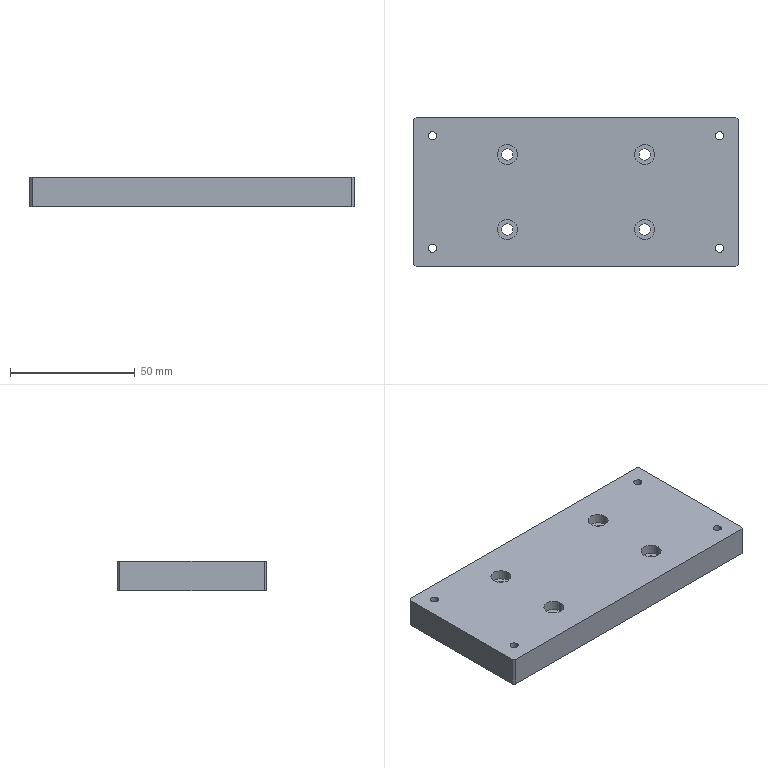Part | NX | features BREP 1 | 1 solid | 38 faces | box 130 x 60 x 12 mm | volume 91852 mm3 | cylinder 24 | plane 14 | commonest cylinder face diameters 3.3 x8 4.5 x8 8 x8
STEP:
#1=CARTESIAN_POINT('',(-59.15,22.5,-6.));
#2=VERTEX_POINT('',#1);
#3=CARTESIAN_POINT('',(-55.85,22.5,-6.));
#4=VERTEX_POINT('',#3);
#5=CARTESIAN_POINT('',(-57.5,22.5,-6.));
#6=DIRECTION('',(0.,0.,1.));
#7=DIRECTION('',(1.,0.,0.));
#8=AXIS2_PLACEMENT_3D('',#5,#6,#7);
#9=CIRCLE('',#8,1.65);
#10=EDGE_CURVE('',#2,#4,#9,.T.);
#11=ORIENTED_EDGE('',*,*,#10,.F.);
#12=CARTESIAN_POINT('',(-59.15,22.5,6.));
#13=VERTEX_POINT('',#12);
#14=CARTESIAN_POINT('',(-59.15,22.5,6.));
#15=DIRECTION('',(0.,0.,1.));
#16=VECTOR('',#15,1000.);
#17=LINE('',#14,#16);
#18=EDGE_CURVE('',#13,#2,#17,.F.);
#19=ORIENTED_EDGE('',*,*,#18,.F.);
#20=CARTESIAN_POINT('',(-55.85,22.5,6.));
#21=VERTEX_POINT('',#20);
#22=CARTESIAN_POINT('',(-57.5,22.5,6.));
#23=DIRECTION('',(0.,0.,1.));
#24=DIRECTION('',(1.,0.,0.));
#25=AXIS2_PLACEMENT_3D('',#22,#23,#24);
#26=CIRCLE('',#25,1.65);
#27=EDGE_CURVE('',#13,#21,#26,.T.);
#28=ORIENTED_EDGE('',*,*,#27,.T.);
#29=CARTESIAN_POINT('',(-55.85,22.5,6.));
#30=DIRECTION('',(0.,0.,1.));
#31=VECTOR('',#30,1000.);
#32=LINE('',#29,#31);
#33=EDGE_CURVE('',#21,#4,#32,.F.);
#34=ORIENTED_EDGE('',*,*,#33,.T.);
#35=EDGE_LOOP('',(#11,#19,#28,#34));
#36=FACE_BOUND('',#35,.T.);
#37=CARTESIAN_POINT('',(-57.5,22.5,6.));
#38=DIRECTION('',(0.,0.,1.));
#39=DIRECTION('',(1.,0.,0.));
#40=AXIS2_PLACEMENT_3D('',#37,#38,#39);
#41=CYLINDRICAL_SURFACE('',#40,1.65);
#42=ADVANCED_FACE('',(#36),#41,.F.);
#43=CARTESIAN_POINT('',(55.85,22.5,-6.));
#44=VERTEX_POINT('',#43);
#45=CARTESIAN_POINT('',(59.15,22.5,-6.));
#46=VERTEX_POINT('',#45);
#47=CARTESIAN_POINT('',(57.5,22.5,-6.));
#48=DIRECTION('',(0.,0.,1.));
#49=DIRECTION('',(1.,0.,0.));
#50=AXIS2_PLACEMENT_3D('',#47,#48,#49);
#51=CIRCLE('',#50,1.65);
#52=EDGE_CURVE('',#44,#46,#51,.T.);
#53=ORIENTED_EDGE('',*,*,#52,.F.);
#54=CARTESIAN_POINT('',(55.85,22.5,6.));
#55=VERTEX_POINT('',#54);
#56=CARTESIAN_POINT('',(55.85,22.5,6.));
#57=DIRECTION('',(0.,0.,1.));
#58=VECTOR('',#57,1000.);
#59=LINE('',#56,#58);
#60=EDGE_CURVE('',#55,#44,#59,.F.);
#61=ORIENTED_EDGE('',*,*,#60,.F.);
#62=CARTESIAN_POINT('',(59.15,22.5,6.));
#63=VERTEX_POINT('',#62);
#64=CARTESIAN_POINT('',(57.5,22.5,6.));
#65=DIRECTION('',(0.,0.,1.));
#66=DIRECTION('',(1.,0.,0.));
#67=AXIS2_PLACEMENT_3D('',#64,#65,#66);
#68=CIRCLE('',#67,1.65);
#69=EDGE_CURVE('',#55,#63,#68,.T.);
#70=ORIENTED_EDGE('',*,*,#69,.T.);
#71=CARTESIAN_POINT('',(59.15,22.5,6.));
#72=DIRECTION('',(0.,0.,1.));
#73=VECTOR('',#72,1000.);
#74=LINE('',#71,#73);
#75=EDGE_CURVE('',#63,#46,#74,.F.);
#76=ORIENTED_EDGE('',*,*,#75,.T.);
#77=EDGE_LOOP('',(#53,#61,#70,#76));
#78=FACE_BOUND('',#77,.T.);
#79=CARTESIAN_POINT('',(57.5,22.5,6.));
#80=DIRECTION('',(0.,0.,1.));
#81=DIRECTION('',(1.,0.,0.));
#82=AXIS2_PLACEMENT_3D('',#79,#80,#81);
#83=CYLINDRICAL_SURFACE('',#82,1.65);
#84=ADVANCED_FACE('',(#78),#83,.F.);
#85=CARTESIAN_POINT('',(-59.15,-22.5,-6.));
#86=VERTEX_POINT('',#85);
#87=CARTESIAN_POINT('',(-55.85,-22.5,-6.));
#88=VERTEX_POINT('',#87);
#89=CARTESIAN_POINT('',(-57.5,-22.5,-6.));
#90=DIRECTION('',(0.,0.,1.));
#91=DIRECTION('',(1.,0.,0.));
#92=AXIS2_PLACEMENT_3D('',#89,#90,#91);
#93=CIRCLE('',#92,1.65);
#94=EDGE_CURVE('',#86,#88,#93,.T.);
#95=ORIENTED_EDGE('',*,*,#94,.F.);
#96=CARTESIAN_POINT('',(-59.15,-22.5,6.));
#97=VERTEX_POINT('',#96);
#98=CARTESIAN_POINT('',(-59.15,-22.5,6.));
#99=DIRECTION('',(0.,0.,1.));
#100=VECTOR('',#99,1000.);
#101=LINE('',#98,#100);
#102=EDGE_CURVE('',#97,#86,#101,.F.);
#103=ORIENTED_EDGE('',*,*,#102,.F.);
#104=CARTESIAN_POINT('',(-55.85,-22.5,6.));
#105=VERTEX_POINT('',#104);
#106=CARTESIAN_POINT('',(-57.5,-22.5,6.));
#107=DIRECTION('',(0.,0.,1.));
#108=DIRECTION('',(1.,0.,0.));
#109=AXIS2_PLACEMENT_3D('',#106,#107,#108);
#110=CIRCLE('',#109,1.65);
#111=EDGE_CURVE('',#97,#105,#110,.T.);
#112=ORIENTED_EDGE('',*,*,#111,.T.);
#113=CARTESIAN_POINT('',(-55.85,-22.5,6.));
#114=DIRECTION('',(0.,0.,1.));
#115=VECTOR('',#114,1000.);
#116=LINE('',#113,#115);
#117=EDGE_CURVE('',#105,#88,#116,.F.);
#118=ORIENTED_EDGE('',*,*,#117,.T.);
#119=EDGE_LOOP('',(#95,#103,#112,#118));
#120=FACE_BOUND('',#119,.T.);
#121=CARTESIAN_POINT('',(-57.5,-22.5,6.));
#122=DIRECTION('',(0.,0.,1.));
#123=DIRECTION('',(1.,0.,0.));
#124=AXIS2_PLACEMENT_3D('',#121,#122,#123);
#125=CYLINDRICAL_SURFACE('',#124,1.65);
#126=ADVANCED_FACE('',(#120),#125,.F.);
#127=CARTESIAN_POINT('',(55.85,-22.5,-6.));
#128=VERTEX_POINT('',#127);
#129=CARTESIAN_POINT('',(59.15,-22.5,-6.));
#130=VERTEX_POINT('',#129);
#131=CARTESIAN_POINT('',(57.5,-22.5,-6.));
#132=DIRECTION('',(0.,0.,1.));
#133=DIRECTION('',(1.,0.,0.));
#134=AXIS2_PLACEMENT_3D('',#131,#132,#133);
#135=CIRCLE('',#134,1.65);
#136=EDGE_CURVE('',#128,#130,#135,.T.);
#137=ORIENTED_EDGE('',*,*,#136,.F.);
#138=CARTESIAN_POINT('',(55.85,-22.5,6.));
#139=VERTEX_POINT('',#138);
#140=CARTESIAN_POINT('',(55.85,-22.5,6.));
#141=DIRECTION('',(0.,0.,1.));
#142=VECTOR('',#141,1000.);
#143=LINE('',#140,#142);
#144=EDGE_CURVE('',#139,#128,#143,.F.);
#145=ORIENTED_EDGE('',*,*,#144,.F.);
#146=CARTESIAN_POINT('',(59.15,-22.5,6.));
#147=VERTEX_POINT('',#146);
#148=CARTESIAN_POINT('',(57.5,-22.5,6.));
#149=DIRECTION('',(0.,0.,1.));
#150=DIRECTION('',(1.,0.,0.));
#151=AXIS2_PLACEMENT_3D('',#148,#149,#150);
#152=CIRCLE('',#151,1.65);
#153=EDGE_CURVE('',#139,#147,#152,.T.);
#154=ORIENTED_EDGE('',*,*,#153,.T.);
#155=CARTESIAN_POINT('',(59.15,-22.5,6.));
#156=DIRECTION('',(0.,0.,1.));
#157=VECTOR('',#156,1000.);
#158=LINE('',#155,#157);
#159=EDGE_CURVE('',#147,#130,#158,.F.);
#160=ORIENTED_EDGE('',*,*,#159,.T.);
#161=EDGE_LOOP('',(#137,#145,#154,#160));
#162=FACE_BOUND('',#161,.T.);
#163=CARTESIAN_POINT('',(57.5,-22.5,6.));
#164=DIRECTION('',(0.,0.,1.));
#165=DIRECTION('',(1.,0.,0.));
#166=AXIS2_PLACEMENT_3D('',#163,#164,#165);
#167=CYLINDRICAL_SURFACE('',#166,1.65);
#168=ADVANCED_FACE('',(#162),#167,.F.);
#169=CARTESIAN_POINT('',(-31.5,15.,2.));
#170=VERTEX_POINT('',#169);
#171=CARTESIAN_POINT('',(-23.5,15.,2.));
#172=VERTEX_POINT('',#171);
#173=CARTESIAN_POINT('',(-27.5,15.,2.));
#174=DIRECTION('',(0.,0.,1.));
#175=DIRECTION('',(1.,0.,0.));
#176=AXIS2_PLACEMENT_3D('',#173,#174,#175);
#177=CIRCLE('',#176,4.);
#178=EDGE_CURVE('',#170,#172,#177,.T.);
#179=ORIENTED_EDGE('',*,*,#178,.F.);
#180=CARTESIAN_POINT('',(-31.5,15.,6.));
#181=VERTEX_POINT('',#180);
#182=CARTESIAN_POINT('',(-31.5,15.,6.));
#183=DIRECTION('',(0.,0.,1.));
#184=VECTOR('',#183,1000.);
#185=LINE('',#182,#184);
#186=EDGE_CURVE('',#181,#170,#185,.F.);
#187=ORIENTED_EDGE('',*,*,#186,.F.);
#188=CARTESIAN_POINT('',(-23.5,15.,6.));
#189=VERTEX_POINT('',#188);
#190=CARTESIAN_POINT('',(-27.5,15.,6.));
#191=DIRECTION('',(0.,0.,1.));
#192=DIRECTION('',(1.,0.,0.));
#193=AXIS2_PLACEMENT_3D('',#190,#191,#192);
#194=CIRCLE('',#193,4.);
#195=EDGE_CURVE('',#181,#189,#194,.T.);
#196=ORIENTED_EDGE('',*,*,#195,.T.);
#197=CARTESIAN_POINT('',(-23.5,15.,6.));
#198=DIRECTION('',(0.,0.,1.));
#199=VECTOR('',#198,1000.);
#200=LINE('',#197,#199);
#201=EDGE_CURVE('',#189,#172,#200,.F.);
#202=ORIENTED_EDGE('',*,*,#201,.T.);
#203=EDGE_LOOP('',(#179,#187,#196,#202));
#204=FACE_BOUND('',#203,.T.);
#205=CARTESIAN_POINT('',(-27.5,15.,6.));
#206=DIRECTION('',(0.,0.,1.));
#207=DIRECTION('',(1.,0.,0.));
#208=AXIS2_PLACEMENT_3D('',#205,#206,#207);
#209=CYLINDRICAL_SURFACE('',#208,4.);
#210=ADVANCED_FACE('',(#204),#209,.F.);
#211=CARTESIAN_POINT('',(-29.75,15.,-6.));
#212=VERTEX_POINT('',#211);
#213=CARTESIAN_POINT('',(-25.25,15.,-6.));
#214=VERTEX_POINT('',#213);
#215=CARTESIAN_POINT('',(-27.5,15.,-6.));
#216=DIRECTION('',(0.,0.,1.));
#217=DIRECTION('',(1.,0.,0.));
#218=AXIS2_PLACEMENT_3D('',#215,#216,#217);
#219=CIRCLE('',#218,2.25);
#220=EDGE_CURVE('',#212,#214,#219,.T.);
#221=ORIENTED_EDGE('',*,*,#220,.F.);
#222=CARTESIAN_POINT('',(-29.75,15.,2.));
#223=VERTEX_POINT('',#222);
#224=CARTESIAN_POINT('',(-29.75,15.,6.));
#225=DIRECTION('',(0.,0.,1.));
#226=VECTOR('',#225,1000.);
#227=LINE('',#224,#226);
#228=EDGE_CURVE('',#223,#212,#227,.F.);
#229=ORIENTED_EDGE('',*,*,#228,.F.);
#230=CARTESIAN_POINT('',(-25.25,15.,2.));
#231=VERTEX_POINT('',#230);
#232=CARTESIAN_POINT('',(-27.5,15.,2.));
#233=DIRECTION('',(0.,0.,1.));
#234=DIRECTION('',(1.,0.,0.));
#235=AXIS2_PLACEMENT_3D('',#232,#233,#234);
#236=CIRCLE('',#235,2.25);
#237=EDGE_CURVE('',#223,#231,#236,.T.);
#238=ORIENTED_EDGE('',*,*,#237,.T.);
#239=CARTESIAN_POINT('',(-25.25,15.,6.));
#240=DIRECTION('',(0.,0.,1.));
#241=VECTOR('',#240,1000.);
#242=LINE('',#239,#241);
#243=EDGE_CURVE('',#231,#214,#242,.F.);
#244=ORIENTED_EDGE('',*,*,#243,.T.);
#245=EDGE_LOOP('',(#221,#229,#238,#244));
#246=FACE_BOUND('',#245,.T.);
#247=CARTESIAN_POINT('',(-27.5,15.,6.));
#248=DIRECTION('',(0.,0.,1.));
#249=DIRECTION('',(1.,0.,0.));
#250=AXIS2_PLACEMENT_3D('',#247,#248,#249);
#251=CYLINDRICAL_SURFACE('',#250,2.25);
#252=ADVANCED_FACE('',(#246),#251,.F.);
#253=CARTESIAN_POINT('',(23.5,15.,2.));
#254=VERTEX_POINT('',#253);
#255=CARTESIAN_POINT('',(31.5,15.,2.));
#256=VERTEX_POINT('',#255);
#257=CARTESIAN_POINT('',(27.5,15.,2.));
#258=DIRECTION('',(0.,0.,1.));
#259=DIRECTION('',(1.,0.,0.));
#260=AXIS2_PLACEMENT_3D('',#257,#258,#259);
#261=CIRCLE('',#260,4.);
#262=EDGE_CURVE('',#254,#256,#261,.T.);
#263=ORIENTED_EDGE('',*,*,#262,.F.);
#264=CARTESIAN_POINT('',(23.5,15.,6.));
#265=VERTEX_POINT('',#264);
#266=CARTESIAN_POINT('',(23.5,15.,6.));
#267=DIRECTION('',(0.,0.,1.));
#268=VECTOR('',#267,1000.);
#269=LINE('',#266,#268);
#270=EDGE_CURVE('',#265,#254,#269,.F.);
#271=ORIENTED_EDGE('',*,*,#270,.F.);
#272=CARTESIAN_POINT('',(31.5,15.,6.));
#273=VERTEX_POINT('',#272);
#274=CARTESIAN_POINT('',(27.5,15.,6.));
#275=DIRECTION('',(0.,0.,1.));
#276=DIRECTION('',(1.,0.,0.));
#277=AXIS2_PLACEMENT_3D('',#274,#275,#276);
#278=CIRCLE('',#277,4.);
#279=EDGE_CURVE('',#265,#273,#278,.T.);
#280=ORIENTED_EDGE('',*,*,#279,.T.);
#281=CARTESIAN_POINT('',(31.5,15.,6.));
#282=DIRECTION('',(0.,0.,1.));
#283=VECTOR('',#282,1000.);
#284=LINE('',#281,#283);
#285=EDGE_CURVE('',#273,#256,#284,.F.);
#286=ORIENTED_EDGE('',*,*,#285,.T.);
#287=EDGE_LOOP('',(#263,#271,#280,#286));
#288=FACE_BOUND('',#287,.T.);
#289=CARTESIAN_POINT('',(27.5,15.,6.));
#290=DIRECTION('',(0.,0.,1.));
#291=DIRECTION('',(1.,0.,0.));
#292=AXIS2_PLACEMENT_3D('',#289,#290,#291);
#293=CYLINDRICAL_SURFACE('',#292,4.);
#294=ADVANCED_FACE('',(#288),#293,.F.);
#295=CARTESIAN_POINT('',(25.25,15.,-6.));
#296=VERTEX_POINT('',#295);
#297=CARTESIAN_POINT('',(29.75,15.,-6.));
#298=VERTEX_POINT('',#297);
#299=CARTESIAN_POINT('',(27.5,15.,-6.));
#300=DIRECTION('',(0.,0.,1.));
#301=DIRECTION('',(1.,0.,0.));
#302=AXIS2_PLACEMENT_3D('',#299,#300,#301);
#303=CIRCLE('',#302,2.25);
#304=EDGE_CURVE('',#296,#298,#303,.T.);
#305=ORIENTED_EDGE('',*,*,#304,.F.);
#306=CARTESIAN_POINT('',(25.25,15.,2.));
#307=VERTEX_POINT('',#306);
#308=CARTESIAN_POINT('',(25.25,15.,6.));
#309=DIRECTION('',(0.,0.,1.));
#310=VECTOR('',#309,1000.);
#311=LINE('',#308,#310);
#312=EDGE_CURVE('',#307,#296,#311,.F.);
#313=ORIENTED_EDGE('',*,*,#312,.F.);
#314=CARTESIAN_POINT('',(29.75,15.,2.));
#315=VERTEX_POINT('',#314);
#316=CARTESIAN_POINT('',(27.5,15.,2.));
#317=DIRECTION('',(0.,0.,1.));
#318=DIRECTION('',(1.,0.,0.));
#319=AXIS2_PLACEMENT_3D('',#316,#317,#318);
#320=CIRCLE('',#319,2.25);
#321=EDGE_CURVE('',#307,#315,#320,.T.);
#322=ORIENTED_EDGE('',*,*,#321,.T.);
#323=CARTESIAN_POINT('',(29.75,15.,6.));
#324=DIRECTION('',(0.,0.,1.));
#325=VECTOR('',#324,1000.);
#326=LINE('',#323,#325);
#327=EDGE_CURVE('',#315,#298,#326,.F.);
#328=ORIENTED_EDGE('',*,*,#327,.T.);
#329=EDGE_LOOP('',(#305,#313,#322,#328));
#330=FACE_BOUND('',#329,.T.);
#331=CARTESIAN_POINT('',(27.5,15.,6.));
#332=DIRECTION('',(0.,0.,1.));
#333=DIRECTION('',(1.,0.,0.));
#334=AXIS2_PLACEMENT_3D('',#331,#332,#333);
#335=CYLINDRICAL_SURFACE('',#334,2.25);
#336=ADVANCED_FACE('',(#330),#335,.F.);
#337=CARTESIAN_POINT('',(-31.5,-15.,2.));
#338=VERTEX_POINT('',#337);
#339=CARTESIAN_POINT('',(-23.5,-15.,2.));
#340=VERTEX_POINT('',#339);
#341=CARTESIAN_POINT('',(-27.5,-15.,2.));
#342=DIRECTION('',(0.,0.,1.));
#343=DIRECTION('',(1.,0.,0.));
#344=AXIS2_PLACEMENT_3D('',#341,#342,#343);
#345=CIRCLE('',#344,4.);
#346=EDGE_CURVE('',#338,#340,#345,.T.);
#347=ORIENTED_EDGE('',*,*,#346,.F.);
#348=CARTESIAN_POINT('',(-31.5,-15.,6.));
#349=VERTEX_POINT('',#348);
#350=CARTESIAN_POINT('',(-31.5,-15.,6.));
#351=DIRECTION('',(0.,0.,1.));
#352=VECTOR('',#351,1000.);
#353=LINE('',#350,#352);
#354=EDGE_CURVE('',#349,#338,#353,.F.);
#355=ORIENTED_EDGE('',*,*,#354,.F.);
#356=CARTESIAN_POINT('',(-23.5,-15.,6.));
#357=VERTEX_POINT('',#356);
#358=CARTESIAN_POINT('',(-27.5,-15.,6.));
#359=DIRECTION('',(0.,0.,1.));
#360=DIRECTION('',(1.,0.,0.));
#361=AXIS2_PLACEMENT_3D('',#358,#359,#360);
#362=CIRCLE('',#361,4.);
#363=EDGE_CURVE('',#349,#357,#362,.T.);
#364=ORIENTED_EDGE('',*,*,#363,.T.);
#365=CARTESIAN_POINT('',(-23.5,-15.,6.));
#366=DIRECTION('',(0.,0.,1.));
#367=VECTOR('',#366,1000.);
#368=LINE('',#365,#367);
#369=EDGE_CURVE('',#357,#340,#368,.F.);
#370=ORIENTED_EDGE('',*,*,#369,.T.);
#371=EDGE_LOOP('',(#347,#355,#364,#370));
#372=FACE_BOUND('',#371,.T.);
#373=CARTESIAN_POINT('',(-27.5,-15.,6.));
#374=DIRECTION('',(0.,0.,1.));
#375=DIRECTION('',(1.,0.,0.));
#376=AXIS2_PLACEMENT_3D('',#373,#374,#375);
#377=CYLINDRICAL_SURFACE('',#376,4.);
#378=ADVANCED_FACE('',(#372),#377,.F.);
#379=CARTESIAN_POINT('',(-29.75,-15.,-6.));
#380=VERTEX_POINT('',#379);
#381=CARTESIAN_POINT('',(-25.25,-15.,-6.));
#382=VERTEX_POINT('',#381);
#383=CARTESIAN_POINT('',(-27.5,-15.,-6.));
#384=DIRECTION('',(0.,0.,1.));
#385=DIRECTION('',(1.,0.,0.));
#386=AXIS2_PLACEMENT_3D('',#383,#384,#385);
#387=CIRCLE('',#386,2.25);
#388=EDGE_CURVE('',#380,#382,#387,.T.);
#389=ORIENTED_EDGE('',*,*,#388,.F.);
#390=CARTESIAN_POINT('',(-29.75,-15.,2.));
#391=VERTEX_POINT('',#390);
#392=CARTESIAN_POINT('',(-29.75,-15.,6.));
#393=DIRECTION('',(0.,0.,1.));
#394=VECTOR('',#393,1000.);
#395=LINE('',#392,#394);
#396=EDGE_CURVE('',#391,#380,#395,.F.);
#397=ORIENTED_EDGE('',*,*,#396,.F.);
#398=CARTESIAN_POINT('',(-25.25,-15.,2.));
#399=VERTEX_POINT('',#398);
#400=CARTESIAN_POINT('',(-27.5,-15.,2.));
#401=DIRECTION('',(0.,0.,1.));
#402=DIRECTION('',(1.,0.,0.));
#403=AXIS2_PLACEMENT_3D('',#400,#401,#402);
#404=CIRCLE('',#403,2.25);
#405=EDGE_CURVE('',#391,#399,#404,.T.);
#406=ORIENTED_EDGE('',*,*,#405,.T.);
#407=CARTESIAN_POINT('',(-25.25,-15.,6.));
#408=DIRECTION('',(0.,0.,1.));
#409=VECTOR('',#408,1000.);
#410=LINE('',#407,#409);
#411=EDGE_CURVE('',#399,#382,#410,.F.);
#412=ORIENTED_EDGE('',*,*,#411,.T.);
#413=EDGE_LOOP('',(#389,#397,#406,#412));
#414=FACE_BOUND('',#413,.T.);
#415=CARTESIAN_POINT('',(-27.5,-15.,6.));
#416=DIRECTION('',(0.,0.,1.));
#417=DIRECTION('',(1.,0.,0.));
#418=AXIS2_PLACEMENT_3D('',#415,#416,#417);
#419=CYLINDRICAL_SURFACE('',#418,2.25);
#420=ADVANCED_FACE('',(#414),#419,.F.);
#421=CARTESIAN_POINT('',(23.5,-15.,2.));
#422=VERTEX_POINT('',#421);
#423=CARTESIAN_POINT('',(31.5,-15.,2.));
#424=VERTEX_POINT('',#423);
#425=CARTESIAN_POINT('',(27.5,-15.,2.));
#426=DIRECTION('',(0.,0.,1.));
#427=DIRECTION('',(1.,0.,0.));
#428=AXIS2_PLACEMENT_3D('',#425,#426,#427);
#429=CIRCLE('',#428,4.);
#430=EDGE_CURVE('',#422,#424,#429,.T.);
#431=ORIENTED_EDGE('',*,*,#430,.F.);
#432=CARTESIAN_POINT('',(23.5,-15.,6.));
#433=VERTEX_POINT('',#432);
#434=CARTESIAN_POINT('',(23.5,-15.,6.));
#435=DIRECTION('',(0.,0.,1.));
#436=VECTOR('',#435,1000.);
#437=LINE('',#434,#436);
#438=EDGE_CURVE('',#433,#422,#437,.F.);
#439=ORIENTED_EDGE('',*,*,#438,.F.);
#440=CARTESIAN_POINT('',(31.5,-15.,6.));
#441=VERTEX_POINT('',#440);
#442=CARTESIAN_POINT('',(27.5,-15.,6.));
#443=DIRECTION('',(0.,0.,1.));
#444=DIRECTION('',(1.,0.,0.));
#445=AXIS2_PLACEMENT_3D('',#442,#443,#444);
#446=CIRCLE('',#445,4.);
#447=EDGE_CURVE('',#433,#441,#446,.T.);
#448=ORIENTED_EDGE('',*,*,#447,.T.);
#449=CARTESIAN_POINT('',(31.5,-15.,6.));
#450=DIRECTION('',(0.,0.,1.));
#451=VECTOR('',#450,1000.);
#452=LINE('',#449,#451);
#453=EDGE_CURVE('',#441,#424,#452,.F.);
#454=ORIENTED_EDGE('',*,*,#453,.T.);
#455=EDGE_LOOP('',(#431,#439,#448,#454));
#456=FACE_BOUND('',#455,.T.);
#457=CARTESIAN_POINT('',(27.5,-15.,6.));
#458=DIRECTION('',(0.,0.,1.));
#459=DIRECTION('',(1.,0.,0.));
#460=AXIS2_PLACEMENT_3D('',#457,#458,#459);
#461=CYLINDRICAL_SURFACE('',#460,4.);
#462=ADVANCED_FACE('',(#456),#461,.F.);
#463=CARTESIAN_POINT('',(25.25,-15.,-6.));
#464=VERTEX_POINT('',#463);
#465=CARTESIAN_POINT('',(29.75,-15.,-6.));
#466=VERTEX_POINT('',#465);
#467=CARTESIAN_POINT('',(27.5,-15.,-6.));
#468=DIRECTION('',(0.,0.,1.));
#469=DIRECTION('',(1.,0.,0.));
#470=AXIS2_PLACEMENT_3D('',#467,#468,#469);
#471=CIRCLE('',#470,2.25);
#472=EDGE_CURVE('',#464,#466,#471,.T.);
#473=ORIENTED_EDGE('',*,*,#472,.F.);
#474=CARTESIAN_POINT('',(25.25,-15.,2.));
#475=VERTEX_POINT('',#474);
#476=CARTESIAN_POINT('',(25.25,-15.,6.));
#477=DIRECTION('',(0.,0.,1.));
#478=VECTOR('',#477,1000.);
#479=LINE('',#476,#478);
#480=EDGE_CURVE('',#475,#464,#479,.F.);
#481=ORIENTED_EDGE('',*,*,#480,.F.);
#482=CARTESIAN_POINT('',(29.75,-15.,2.));
#483=VERTEX_POINT('',#482);
#484=CARTESIAN_POINT('',(27.5,-15.,2.));
#485=DIRECTION('',(0.,0.,1.));
#486=DIRECTION('',(1.,0.,0.));
#487=AXIS2_PLACEMENT_3D('',#484,#485,#486);
#488=CIRCLE('',#487,2.25);
#489=EDGE_CURVE('',#475,#483,#488,.T.);
#490=ORIENTED_EDGE('',*,*,#489,.T.);
#491=CARTESIAN_POINT('',(29.75,-15.,6.));
#492=DIRECTION('',(0.,0.,1.));
#493=VECTOR('',#492,1000.);
#494=LINE('',#491,#493);
#495=EDGE_CURVE('',#483,#466,#494,.F.);
#496=ORIENTED_EDGE('',*,*,#495,.T.);
#497=EDGE_LOOP('',(#473,#481,#490,#496));
#498=FACE_BOUND('',#497,.T.);
#499=CARTESIAN_POINT('',(27.5,-15.,6.));
#500=DIRECTION('',(0.,0.,1.));
#501=DIRECTION('',(1.,0.,0.));
#502=AXIS2_PLACEMENT_3D('',#499,#500,#501);
#503=CYLINDRICAL_SURFACE('',#502,2.25);
#504=ADVANCED_FACE('',(#498),#503,.F.);
#505=CARTESIAN_POINT('',(-65.,29.,-6.));
#506=VERTEX_POINT('',#505);
#507=CARTESIAN_POINT('',(-65.,-29.,-6.));
#508=VERTEX_POINT('',#507);
#509=CARTESIAN_POINT('',(-65.,-30.,-6.));
#510=DIRECTION('',(0.,-1.,0.));
#511=VECTOR('',#510,1000.);
#512=LINE('',#509,#511);
#513=EDGE_CURVE('',#506,#508,#512,.T.);
#514=ORIENTED_EDGE('',*,*,#513,.T.);
#515=CARTESIAN_POINT('',(-65.,-29.,6.));
#516=VERTEX_POINT('',#515);
#517=CARTESIAN_POINT('',(-65.,-29.,6.));
#518=DIRECTION('',(0.,0.,1.));
#519=VECTOR('',#518,1000.);
#520=LINE('',#517,#519);
#521=EDGE_CURVE('',#508,#516,#520,.T.);
#522=ORIENTED_EDGE('',*,*,#521,.T.);
#523=CARTESIAN_POINT('',(-65.,29.,6.));
#524=VERTEX_POINT('',#523);
#525=CARTESIAN_POINT('',(-65.,-30.,6.));
#526=DIRECTION('',(0.,-1.,0.));
#527=VECTOR('',#526,1000.);
#528=LINE('',#525,#527);
#529=EDGE_CURVE('',#524,#516,#528,.T.);
#530=ORIENTED_EDGE('',*,*,#529,.F.);
#531=CARTESIAN_POINT('',(-65.,29.,6.));
#532=DIRECTION('',(0.,0.,-1.));
#533=VECTOR('',#532,1000.);
#534=LINE('',#531,#533);
#535=EDGE_CURVE('',#524,#506,#534,.T.);
#536=ORIENTED_EDGE('',*,*,#535,.T.);
#537=EDGE_LOOP('',(#514,#522,#530,#536));
#538=FACE_BOUND('',#537,.T.);
#539=CARTESIAN_POINT('',(-65.,-30.,6.));
#540=DIRECTION('',(1.,0.,0.));
#541=DIRECTION('',(0.,1.,0.));
#542=AXIS2_PLACEMENT_3D('',#539,#540,#541);
#543=PLANE('',#542);
#544=ADVANCED_FACE('',(#538),#543,.F.);
#545=CARTESIAN_POINT('',(-64.,-30.,6.));
#546=VERTEX_POINT('',#545);
#547=CARTESIAN_POINT('',(64.,-30.,6.));
#548=VERTEX_POINT('',#547);
#549=CARTESIAN_POINT('',(65.,-30.,6.));
#550=DIRECTION('',(1.,0.,0.));
#551=VECTOR('',#550,1000.);
#552=LINE('',#549,#551);
#553=EDGE_CURVE('',#546,#548,#552,.T.);
#554=ORIENTED_EDGE('',*,*,#553,.F.);
#555=CARTESIAN_POINT('',(-64.,-30.,-6.));
#556=VERTEX_POINT('',#555);
#557=CARTESIAN_POINT('',(-64.,-30.,6.));
#558=DIRECTION('',(0.,0.,-1.));
#559=VECTOR('',#558,1000.);
#560=LINE('',#557,#559);
#561=EDGE_CURVE('',#546,#556,#560,.T.);
#562=ORIENTED_EDGE('',*,*,#561,.T.);
#563=CARTESIAN_POINT('',(64.,-30.,-6.));
#564=VERTEX_POINT('',#563);
#565=CARTESIAN_POINT('',(65.,-30.,-6.));
#566=DIRECTION('',(1.,0.,0.));
#567=VECTOR('',#566,1000.);
#568=LINE('',#565,#567);
#569=EDGE_CURVE('',#556,#564,#568,.T.);
#570=ORIENTED_EDGE('',*,*,#569,.T.);
#571=CARTESIAN_POINT('',(64.,-30.,6.));
#572=DIRECTION('',(0.,0.,1.));
#573=VECTOR('',#572,1000.);
#574=LINE('',#571,#573);
#575=EDGE_CURVE('',#564,#548,#574,.T.);
#576=ORIENTED_EDGE('',*,*,#575,.T.);
#577=EDGE_LOOP('',(#554,#562,#570,#576));
#578=FACE_BOUND('',#577,.T.);
#579=CARTESIAN_POINT('',(65.,-30.,6.));
#580=DIRECTION('',(0.,1.,0.));
#581=DIRECTION('',(1.,0.,0.));
#582=AXIS2_PLACEMENT_3D('',#579,#580,#581);
#583=PLANE('',#582);
#584=ADVANCED_FACE('',(#578),#583,.F.);
#585=CARTESIAN_POINT('',(65.,-29.,6.));
#586=VERTEX_POINT('',#585);
#587=CARTESIAN_POINT('',(65.,29.,6.));
#588=VERTEX_POINT('',#587);
#589=CARTESIAN_POINT('',(65.,-30.,6.));
#590=DIRECTION('',(0.,1.,0.));
#591=VECTOR('',#590,1000.);
#592=LINE('',#589,#591);
#593=EDGE_CURVE('',#586,#588,#592,.T.);
#594=ORIENTED_EDGE('',*,*,#593,.F.);
#595=CARTESIAN_POINT('',(65.,-29.,-6.));
#596=VERTEX_POINT('',#595);
#597=CARTESIAN_POINT('',(65.,-29.,6.));
#598=DIRECTION('',(0.,0.,-1.));
#599=VECTOR('',#598,1000.);
#600=LINE('',#597,#599);
#601=EDGE_CURVE('',#586,#596,#600,.T.);
#602=ORIENTED_EDGE('',*,*,#601,.T.);
#603=CARTESIAN_POINT('',(65.,29.,-6.));
#604=VERTEX_POINT('',#603);
#605=CARTESIAN_POINT('',(65.,-30.,-6.));
#606=DIRECTION('',(0.,1.,0.));
#607=VECTOR('',#606,1000.);
#608=LINE('',#605,#607);
#609=EDGE_CURVE('',#596,#604,#608,.T.);
#610=ORIENTED_EDGE('',*,*,#609,.T.);
#611=CARTESIAN_POINT('',(65.,29.,6.));
#612=DIRECTION('',(0.,0.,1.));
#613=VECTOR('',#612,1000.);
#614=LINE('',#611,#613);
#615=EDGE_CURVE('',#604,#588,#614,.T.);
#616=ORIENTED_EDGE('',*,*,#615,.T.);
#617=EDGE_LOOP('',(#594,#602,#610,#616));
#618=FACE_BOUND('',#617,.T.);
#619=CARTESIAN_POINT('',(65.,-30.,6.));
#620=DIRECTION('',(-1.,0.,0.));
#621=DIRECTION('',(0.,0.,1.));
#622=AXIS2_PLACEMENT_3D('',#619,#620,#621);
#623=PLANE('',#622);
#624=ADVANCED_FACE('',(#618),#623,.F.);
#625=CARTESIAN_POINT('',(64.,30.,-6.));
#626=VERTEX_POINT('',#625);
#627=CARTESIAN_POINT('',(-64.,30.,-6.));
#628=VERTEX_POINT('',#627);
#629=CARTESIAN_POINT('',(65.,30.,-6.));
#630=DIRECTION('',(-1.,0.,0.));
#631=VECTOR('',#630,1000.);
#632=LINE('',#629,#631);
#633=EDGE_CURVE('',#626,#628,#632,.T.);
#634=ORIENTED_EDGE('',*,*,#633,.T.);
#635=CARTESIAN_POINT('',(-64.,30.,6.));
#636=VERTEX_POINT('',#635);
#637=CARTESIAN_POINT('',(-64.,30.,6.));
#638=DIRECTION('',(0.,0.,1.));
#639=VECTOR('',#638,1000.);
#640=LINE('',#637,#639);
#641=EDGE_CURVE('',#628,#636,#640,.T.);
#642=ORIENTED_EDGE('',*,*,#641,.T.);
#643=CARTESIAN_POINT('',(64.,30.,6.));
#644=VERTEX_POINT('',#643);
#645=CARTESIAN_POINT('',(65.,30.,6.));
#646=DIRECTION('',(-1.,0.,0.));
#647=VECTOR('',#646,1000.);
#648=LINE('',#645,#647);
#649=EDGE_CURVE('',#644,#636,#648,.T.);
#650=ORIENTED_EDGE('',*,*,#649,.F.);
#651=CARTESIAN_POINT('',(64.,30.,6.));
#652=DIRECTION('',(0.,0.,-1.));
#653=VECTOR('',#652,1000.);
#654=LINE('',#651,#653);
#655=EDGE_CURVE('',#644,#626,#654,.T.);
#656=ORIENTED_EDGE('',*,*,#655,.T.);
#657=EDGE_LOOP('',(#634,#642,#650,#656));
#658=FACE_BOUND('',#657,.T.);
#659=CARTESIAN_POINT('',(65.,30.,6.));
#660=DIRECTION('',(0.,-1.,0.));
#661=DIRECTION('',(0.,0.,-1.));
#662=AXIS2_PLACEMENT_3D('',#659,#660,#661);
#663=PLANE('',#662);
#664=ADVANCED_FACE('',(#658),#663,.F.);
#665=ORIENTED_EDGE('',*,*,#529,.T.);
#666=CARTESIAN_POINT('',(-47.,-47.,6.));
#667=DIRECTION('',(0.7071,-0.7071,0.));
#668=VECTOR('',#667,1000.);
#669=LINE('',#666,#668);
#670=EDGE_CURVE('',#516,#546,#669,.T.);
#671=ORIENTED_EDGE('',*,*,#670,.T.);
#672=ORIENTED_EDGE('',*,*,#553,.T.);
#673=CARTESIAN_POINT('',(47.,-47.,6.));
#674=DIRECTION('',(0.7071,0.7071,0.));
#675=VECTOR('',#674,1000.);
#676=LINE('',#673,#675);
#677=EDGE_CURVE('',#548,#586,#676,.T.);
#678=ORIENTED_EDGE('',*,*,#677,.T.);
#679=ORIENTED_EDGE('',*,*,#593,.T.);
#680=CARTESIAN_POINT('',(47.,47.,6.));
#681=DIRECTION('',(-0.7071,0.7071,0.));
#682=VECTOR('',#681,1000.);
#683=LINE('',#680,#682);
#684=EDGE_CURVE('',#588,#644,#683,.T.);
#685=ORIENTED_EDGE('',*,*,#684,.T.);
#686=ORIENTED_EDGE('',*,*,#649,.T.);
#687=CARTESIAN_POINT('',(-47.,47.,6.));
#688=DIRECTION('',(-0.7071,-0.7071,0.));
#689=VECTOR('',#688,1000.);
#690=LINE('',#687,#689);
#691=EDGE_CURVE('',#636,#524,#690,.T.);
#692=ORIENTED_EDGE('',*,*,#691,.T.);
#693=EDGE_LOOP('',(#665,#671,#672,#678,#679,#685,#686,#692));
#694=FACE_BOUND('',#693,.T.);
#695=CARTESIAN_POINT('',(-57.5,22.5,6.));
#696=DIRECTION('',(0.,0.,1.));
#697=DIRECTION('',(1.,0.,0.));
#698=AXIS2_PLACEMENT_3D('',#695,#696,#697);
#699=CIRCLE('',#698,1.65);
#700=EDGE_CURVE('',#21,#13,#699,.T.);
#701=ORIENTED_EDGE('',*,*,#700,.F.);
#702=ORIENTED_EDGE('',*,*,#27,.F.);
#703=EDGE_LOOP('',(#701,#702));
#704=FACE_BOUND('',#703,.T.);
#705=CARTESIAN_POINT('',(57.5,22.5,6.));
#706=DIRECTION('',(0.,0.,1.));
#707=DIRECTION('',(1.,0.,0.));
#708=AXIS2_PLACEMENT_3D('',#705,#706,#707);
#709=CIRCLE('',#708,1.65);
#710=EDGE_CURVE('',#63,#55,#709,.T.);
#711=ORIENTED_EDGE('',*,*,#710,.F.);
#712=ORIENTED_EDGE('',*,*,#69,.F.);
#713=EDGE_LOOP('',(#711,#712));
#714=FACE_BOUND('',#713,.T.);
#715=CARTESIAN_POINT('',(-57.5,-22.5,6.));
#716=DIRECTION('',(0.,0.,1.));
#717=DIRECTION('',(1.,0.,0.));
#718=AXIS2_PLACEMENT_3D('',#715,#716,#717);
#719=CIRCLE('',#718,1.65);
#720=EDGE_CURVE('',#105,#97,#719,.T.);
#721=ORIENTED_EDGE('',*,*,#720,.F.);
#722=ORIENTED_EDGE('',*,*,#111,.F.);
#723=EDGE_LOOP('',(#721,#722));
#724=FACE_BOUND('',#723,.T.);
#725=CARTESIAN_POINT('',(57.5,-22.5,6.));
#726=DIRECTION('',(0.,0.,1.));
#727=DIRECTION('',(1.,0.,0.));
#728=AXIS2_PLACEMENT_3D('',#725,#726,#727);
#729=CIRCLE('',#728,1.65);
#730=EDGE_CURVE('',#147,#139,#729,.T.);
#731=ORIENTED_EDGE('',*,*,#730,.F.);
#732=ORIENTED_EDGE('',*,*,#153,.F.);
#733=EDGE_LOOP('',(#731,#732));
#734=FACE_BOUND('',#733,.T.);
#735=CARTESIAN_POINT('',(-27.5,15.,6.));
#736=DIRECTION('',(0.,0.,1.));
#737=DIRECTION('',(1.,0.,0.));
#738=AXIS2_PLACEMENT_3D('',#735,#736,#737);
#739=CIRCLE('',#738,4.);
#740=EDGE_CURVE('',#189,#181,#739,.T.);
#741=ORIENTED_EDGE('',*,*,#740,.F.);
#742=ORIENTED_EDGE('',*,*,#195,.F.);
#743=EDGE_LOOP('',(#741,#742));
#744=FACE_BOUND('',#743,.T.);
#745=CARTESIAN_POINT('',(27.5,15.,6.));
#746=DIRECTION('',(0.,0.,1.));
#747=DIRECTION('',(1.,0.,0.));
#748=AXIS2_PLACEMENT_3D('',#745,#746,#747);
#749=CIRCLE('',#748,4.);
#750=EDGE_CURVE('',#273,#265,#749,.T.);
#751=ORIENTED_EDGE('',*,*,#750,.F.);
#752=ORIENTED_EDGE('',*,*,#279,.F.);
#753=EDGE_LOOP('',(#751,#752));
#754=FACE_BOUND('',#753,.T.);
#755=CARTESIAN_POINT('',(-27.5,-15.,6.));
#756=DIRECTION('',(0.,0.,1.));
#757=DIRECTION('',(1.,0.,0.));
#758=AXIS2_PLACEMENT_3D('',#755,#756,#757);
#759=CIRCLE('',#758,4.);
#760=EDGE_CURVE('',#357,#349,#759,.T.);
#761=ORIENTED_EDGE('',*,*,#760,.F.);
#762=ORIENTED_EDGE('',*,*,#363,.F.);
#763=EDGE_LOOP('',(#761,#762));
#764=FACE_BOUND('',#763,.T.);
#765=CARTESIAN_POINT('',(27.5,-15.,6.));
#766=DIRECTION('',(0.,0.,1.));
#767=DIRECTION('',(1.,0.,0.));
#768=AXIS2_PLACEMENT_3D('',#765,#766,#767);
#769=CIRCLE('',#768,4.);
#770=EDGE_CURVE('',#441,#433,#769,.T.);
#771=ORIENTED_EDGE('',*,*,#770,.F.);
#772=ORIENTED_EDGE('',*,*,#447,.F.);
#773=EDGE_LOOP('',(#771,#772));
#774=FACE_BOUND('',#773,.T.);
#775=CARTESIAN_POINT('',(0.,0.,6.));
#776=DIRECTION('',(0.,0.,1.));
#777=DIRECTION('',(1.,0.,0.));
#778=AXIS2_PLACEMENT_3D('',#775,#776,#777);
#779=PLANE('',#778);
#780=ADVANCED_FACE('',(#694,#704,#714,#724,#734,#744,#754,#764,#774),#779,.T.);
#781=ORIENTED_EDGE('',*,*,#569,.F.);
#782=CARTESIAN_POINT('',(-64.,-30.,-6.));
#783=DIRECTION('',(-0.7071,0.7071,0.));
#784=VECTOR('',#783,1000.);
#785=LINE('',#782,#784);
#786=EDGE_CURVE('',#556,#508,#785,.T.);
#787=ORIENTED_EDGE('',*,*,#786,.T.);
#788=ORIENTED_EDGE('',*,*,#513,.F.);
#789=CARTESIAN_POINT('',(-65.,29.,-6.));
#790=DIRECTION('',(0.7071,0.7071,0.));
#791=VECTOR('',#790,1000.);
#792=LINE('',#789,#791);
#793=EDGE_CURVE('',#506,#628,#792,.T.);
#794=ORIENTED_EDGE('',*,*,#793,.T.);
#795=ORIENTED_EDGE('',*,*,#633,.F.);
#796=CARTESIAN_POINT('',(64.,30.,-6.));
#797=DIRECTION('',(0.7071,-0.7071,0.));
#798=VECTOR('',#797,1000.);
#799=LINE('',#796,#798);
#800=EDGE_CURVE('',#626,#604,#799,.T.);
#801=ORIENTED_EDGE('',*,*,#800,.T.);
#802=ORIENTED_EDGE('',*,*,#609,.F.);
#803=CARTESIAN_POINT('',(65.,-29.,-6.));
#804=DIRECTION('',(-0.7071,-0.7071,0.));
#805=VECTOR('',#804,1000.);
#806=LINE('',#803,#805);
#807=EDGE_CURVE('',#596,#564,#806,.T.);
#808=ORIENTED_EDGE('',*,*,#807,.T.);
#809=EDGE_LOOP('',(#781,#787,#788,#794,#795,#801,#802,#808));
#810=FACE_BOUND('',#809,.T.);
#811=CARTESIAN_POINT('',(-57.5,22.5,-6.));
#812=DIRECTION('',(0.,0.,1.));
#813=DIRECTION('',(1.,0.,0.));
#814=AXIS2_PLACEMENT_3D('',#811,#812,#813);
#815=CIRCLE('',#814,1.65);
#816=EDGE_CURVE('',#4,#2,#815,.T.);
#817=ORIENTED_EDGE('',*,*,#816,.T.);
#818=ORIENTED_EDGE('',*,*,#10,.T.);
#819=EDGE_LOOP('',(#817,#818));
#820=FACE_BOUND('',#819,.T.);
#821=CARTESIAN_POINT('',(57.5,22.5,-6.));
#822=DIRECTION('',(0.,0.,1.));
#823=DIRECTION('',(1.,0.,0.));
#824=AXIS2_PLACEMENT_3D('',#821,#822,#823);
#825=CIRCLE('',#824,1.65);
#826=EDGE_CURVE('',#46,#44,#825,.T.);
#827=ORIENTED_EDGE('',*,*,#826,.T.);
#828=ORIENTED_EDGE('',*,*,#52,.T.);
#829=EDGE_LOOP('',(#827,#828));
#830=FACE_BOUND('',#829,.T.);
#831=CARTESIAN_POINT('',(-57.5,-22.5,-6.));
#832=DIRECTION('',(0.,0.,1.));
#833=DIRECTION('',(1.,0.,0.));
#834=AXIS2_PLACEMENT_3D('',#831,#832,#833);
#835=CIRCLE('',#834,1.65);
#836=EDGE_CURVE('',#88,#86,#835,.T.);
#837=ORIENTED_EDGE('',*,*,#836,.T.);
#838=ORIENTED_EDGE('',*,*,#94,.T.);
#839=EDGE_LOOP('',(#837,#838));
#840=FACE_BOUND('',#839,.T.);
#841=CARTESIAN_POINT('',(57.5,-22.5,-6.));
#842=DIRECTION('',(0.,0.,1.));
#843=DIRECTION('',(1.,0.,0.));
#844=AXIS2_PLACEMENT_3D('',#841,#842,#843);
#845=CIRCLE('',#844,1.65);
#846=EDGE_CURVE('',#130,#128,#845,.T.);
#847=ORIENTED_EDGE('',*,*,#846,.T.);
#848=ORIENTED_EDGE('',*,*,#136,.T.);
#849=EDGE_LOOP('',(#847,#848));
#850=FACE_BOUND('',#849,.T.);
#851=CARTESIAN_POINT('',(-27.5,15.,-6.));
#852=DIRECTION('',(0.,0.,1.));
#853=DIRECTION('',(1.,0.,0.));
#854=AXIS2_PLACEMENT_3D('',#851,#852,#853);
#855=CIRCLE('',#854,2.25);
#856=EDGE_CURVE('',#214,#212,#855,.T.);
#857=ORIENTED_EDGE('',*,*,#856,.T.);
#858=ORIENTED_EDGE('',*,*,#220,.T.);
#859=EDGE_LOOP('',(#857,#858));
#860=FACE_BOUND('',#859,.T.);
#861=CARTESIAN_POINT('',(27.5,15.,-6.));
#862=DIRECTION('',(0.,0.,1.));
#863=DIRECTION('',(1.,0.,0.));
#864=AXIS2_PLACEMENT_3D('',#861,#862,#863);
#865=CIRCLE('',#864,2.25);
#866=EDGE_CURVE('',#298,#296,#865,.T.);
#867=ORIENTED_EDGE('',*,*,#866,.T.);
#868=ORIENTED_EDGE('',*,*,#304,.T.);
#869=EDGE_LOOP('',(#867,#868));
#870=FACE_BOUND('',#869,.T.);
#871=CARTESIAN_POINT('',(-27.5,-15.,-6.));
#872=DIRECTION('',(0.,0.,1.));
#873=DIRECTION('',(1.,0.,0.));
#874=AXIS2_PLACEMENT_3D('',#871,#872,#873);
#875=CIRCLE('',#874,2.25);
#876=EDGE_CURVE('',#382,#380,#875,.T.);
#877=ORIENTED_EDGE('',*,*,#876,.T.);
#878=ORIENTED_EDGE('',*,*,#388,.T.);
#879=EDGE_LOOP('',(#877,#878));
#880=FACE_BOUND('',#879,.T.);
#881=CARTESIAN_POINT('',(27.5,-15.,-6.));
#882=DIRECTION('',(0.,0.,1.));
#883=DIRECTION('',(1.,0.,0.));
#884=AXIS2_PLACEMENT_3D('',#881,#882,#883);
#885=CIRCLE('',#884,2.25);
#886=EDGE_CURVE('',#466,#464,#885,.T.);
#887=ORIENTED_EDGE('',*,*,#886,.T.);
#888=ORIENTED_EDGE('',*,*,#472,.T.);
#889=EDGE_LOOP('',(#887,#888));
#890=FACE_BOUND('',#889,.T.);
#891=CARTESIAN_POINT('',(0.,0.,-6.));
#892=DIRECTION('',(0.,0.,1.));
#893=DIRECTION('',(1.,0.,0.));
#894=AXIS2_PLACEMENT_3D('',#891,#892,#893);
#895=PLANE('',#894);
#896=ADVANCED_FACE('',(#810,#820,#830,#840,#850,#860,#870,#880,#890),#895,.F.);
#897=ORIENTED_EDGE('',*,*,#670,.F.);
#898=ORIENTED_EDGE('',*,*,#521,.F.);
#899=ORIENTED_EDGE('',*,*,#786,.F.);
#900=ORIENTED_EDGE('',*,*,#561,.F.);
#901=EDGE_LOOP('',(#897,#898,#899,#900));
#902=FACE_BOUND('',#901,.T.);
#903=CARTESIAN_POINT('',(-64.,-30.,6.));
#904=DIRECTION('',(0.7071,0.7071,0.));
#905=DIRECTION('',(0.,0.,-1.));
#906=AXIS2_PLACEMENT_3D('',#903,#904,#905);
#907=PLANE('',#906);
#908=ADVANCED_FACE('',(#902),#907,.F.);
#909=ORIENTED_EDGE('',*,*,#691,.F.);
#910=ORIENTED_EDGE('',*,*,#641,.F.);
#911=ORIENTED_EDGE('',*,*,#793,.F.);
#912=ORIENTED_EDGE('',*,*,#535,.F.);
#913=EDGE_LOOP('',(#909,#910,#911,#912));
#914=FACE_BOUND('',#913,.T.);
#915=CARTESIAN_POINT('',(-65.,29.,6.));
#916=DIRECTION('',(0.7071,-0.7071,0.));
#917=DIRECTION('',(0.,0.,-1.));
#918=AXIS2_PLACEMENT_3D('',#915,#916,#917);
#919=PLANE('',#918);
#920=ADVANCED_FACE('',(#914),#919,.F.);
#921=ORIENTED_EDGE('',*,*,#677,.F.);
#922=ORIENTED_EDGE('',*,*,#575,.F.);
#923=ORIENTED_EDGE('',*,*,#807,.F.);
#924=ORIENTED_EDGE('',*,*,#601,.F.);
#925=EDGE_LOOP('',(#921,#922,#923,#924));
#926=FACE_BOUND('',#925,.T.);
#927=CARTESIAN_POINT('',(65.,-29.,6.));
#928=DIRECTION('',(-0.7071,0.7071,0.));
#929=DIRECTION('',(0.,0.,1.));
#930=AXIS2_PLACEMENT_3D('',#927,#928,#929);
#931=PLANE('',#930);
#932=ADVANCED_FACE('',(#926),#931,.F.);
#933=ORIENTED_EDGE('',*,*,#684,.F.);
#934=ORIENTED_EDGE('',*,*,#615,.F.);
#935=ORIENTED_EDGE('',*,*,#800,.F.);
#936=ORIENTED_EDGE('',*,*,#655,.F.);
#937=EDGE_LOOP('',(#933,#934,#935,#936));
#938=FACE_BOUND('',#937,.T.);
#939=CARTESIAN_POINT('',(64.,30.,6.));
#940=DIRECTION('',(-0.7071,-0.7071,0.));
#941=DIRECTION('',(-0.7071,0.7071,0.));
#942=AXIS2_PLACEMENT_3D('',#939,#940,#941);
#943=PLANE('',#942);
#944=ADVANCED_FACE('',(#938),#943,.F.);
#945=ORIENTED_EDGE('',*,*,#480,.T.);
#946=ORIENTED_EDGE('',*,*,#886,.F.);
#947=ORIENTED_EDGE('',*,*,#495,.F.);
#948=CARTESIAN_POINT('',(27.5,-15.,2.));
#949=DIRECTION('',(0.,0.,1.));
#950=DIRECTION('',(1.,0.,0.));
#951=AXIS2_PLACEMENT_3D('',#948,#949,#950);
#952=CIRCLE('',#951,2.25);
#953=EDGE_CURVE('',#483,#475,#952,.T.);
#954=ORIENTED_EDGE('',*,*,#953,.T.);
#955=EDGE_LOOP('',(#945,#946,#947,#954));
#956=FACE_BOUND('',#955,.T.);
#957=CARTESIAN_POINT('',(27.5,-15.,6.));
#958=DIRECTION('',(0.,0.,1.));
#959=DIRECTION('',(1.,0.,0.));
#960=AXIS2_PLACEMENT_3D('',#957,#958,#959);
#961=CYLINDRICAL_SURFACE('',#960,2.25);
#962=ADVANCED_FACE('',(#956),#961,.F.);
#963=CARTESIAN_POINT('',(27.5,-15.,2.));
#964=DIRECTION('',(0.,0.,1.));
#965=DIRECTION('',(1.,0.,0.));
#966=AXIS2_PLACEMENT_3D('',#963,#964,#965);
#967=CIRCLE('',#966,4.);
#968=EDGE_CURVE('',#424,#422,#967,.T.);
#969=ORIENTED_EDGE('',*,*,#968,.T.);
#970=ORIENTED_EDGE('',*,*,#430,.T.);
#971=EDGE_LOOP('',(#969,#970));
#972=FACE_BOUND('',#971,.T.);
#973=ORIENTED_EDGE('',*,*,#953,.F.);
#974=ORIENTED_EDGE('',*,*,#489,.F.);
#975=EDGE_LOOP('',(#973,#974));
#976=FACE_BOUND('',#975,.T.);
#977=CARTESIAN_POINT('',(29.75,-15.,2.));
#978=DIRECTION('',(0.,0.,-1.));
#979=DIRECTION('',(0.,-1.,0.));
#980=AXIS2_PLACEMENT_3D('',#977,#978,#979);
#981=PLANE('',#980);
#982=ADVANCED_FACE('',(#972,#976),#981,.F.);
#983=ORIENTED_EDGE('',*,*,#438,.T.);
#984=ORIENTED_EDGE('',*,*,#968,.F.);
#985=ORIENTED_EDGE('',*,*,#453,.F.);
#986=ORIENTED_EDGE('',*,*,#770,.T.);
#987=EDGE_LOOP('',(#983,#984,#985,#986));
#988=FACE_BOUND('',#987,.T.);
#989=CARTESIAN_POINT('',(27.5,-15.,6.));
#990=DIRECTION('',(0.,0.,1.));
#991=DIRECTION('',(1.,0.,0.));
#992=AXIS2_PLACEMENT_3D('',#989,#990,#991);
#993=CYLINDRICAL_SURFACE('',#992,4.);
#994=ADVANCED_FACE('',(#988),#993,.F.);
#995=ORIENTED_EDGE('',*,*,#396,.T.);
#996=ORIENTED_EDGE('',*,*,#876,.F.);
#997=ORIENTED_EDGE('',*,*,#411,.F.);
#998=CARTESIAN_POINT('',(-27.5,-15.,2.));
#999=DIRECTION('',(0.,0.,1.));
#1000=DIRECTION('',(1.,0.,0.));
#1001=AXIS2_PLACEMENT_3D('',#998,#999,#1000);
#1002=CIRCLE('',#1001,2.25);
#1003=EDGE_CURVE('',#399,#391,#1002,.T.);
#1004=ORIENTED_EDGE('',*,*,#1003,.T.);
#1005=EDGE_LOOP('',(#995,#996,#997,#1004));
#1006=FACE_BOUND('',#1005,.T.);
#1007=CARTESIAN_POINT('',(-27.5,-15.,6.));
#1008=DIRECTION('',(0.,0.,1.));
#1009=DIRECTION('',(1.,0.,0.));
#1010=AXIS2_PLACEMENT_3D('',#1007,#1008,#1009);
#1011=CYLINDRICAL_SURFACE('',#1010,2.25);
#1012=ADVANCED_FACE('',(#1006),#1011,.F.);
#1013=CARTESIAN_POINT('',(-27.5,-15.,2.));
#1014=DIRECTION('',(0.,0.,1.));
#1015=DIRECTION('',(1.,0.,0.));
#1016=AXIS2_PLACEMENT_3D('',#1013,#1014,#1015);
#1017=CIRCLE('',#1016,4.);
#1018=EDGE_CURVE('',#340,#338,#1017,.T.);
#1019=ORIENTED_EDGE('',*,*,#1018,.T.);
#1020=ORIENTED_EDGE('',*,*,#346,.T.);
#1021=EDGE_LOOP('',(#1019,#1020));
#1022=FACE_BOUND('',#1021,.T.);
#1023=ORIENTED_EDGE('',*,*,#1003,.F.);
#1024=ORIENTED_EDGE('',*,*,#405,.F.);
#1025=EDGE_LOOP('',(#1023,#1024));
#1026=FACE_BOUND('',#1025,.T.);
#1027=CARTESIAN_POINT('',(-25.25,-15.,2.));
#1028=DIRECTION('',(0.,0.,-1.));
#1029=DIRECTION('',(0.,-1.,0.));
#1030=AXIS2_PLACEMENT_3D('',#1027,#1028,#1029);
#1031=PLANE('',#1030);
#1032=ADVANCED_FACE('',(#1022,#1026),#1031,.F.);
#1033=ORIENTED_EDGE('',*,*,#354,.T.);
#1034=ORIENTED_EDGE('',*,*,#1018,.F.);
#1035=ORIENTED_EDGE('',*,*,#369,.F.);
#1036=ORIENTED_EDGE('',*,*,#760,.T.);
#1037=EDGE_LOOP('',(#1033,#1034,#1035,#1036));
#1038=FACE_BOUND('',#1037,.T.);
#1039=CARTESIAN_POINT('',(-27.5,-15.,6.));
#1040=DIRECTION('',(0.,0.,1.));
#1041=DIRECTION('',(1.,0.,0.));
#1042=AXIS2_PLACEMENT_3D('',#1039,#1040,#1041);
#1043=CYLINDRICAL_SURFACE('',#1042,4.);
#1044=ADVANCED_FACE('',(#1038),#1043,.F.);
#1045=ORIENTED_EDGE('',*,*,#312,.T.);
#1046=ORIENTED_EDGE('',*,*,#866,.F.);
#1047=ORIENTED_EDGE('',*,*,#327,.F.);
#1048=CARTESIAN_POINT('',(27.5,15.,2.));
#1049=DIRECTION('',(0.,0.,1.));
#1050=DIRECTION('',(1.,0.,0.));
#1051=AXIS2_PLACEMENT_3D('',#1048,#1049,#1050);
#1052=CIRCLE('',#1051,2.25);
#1053=EDGE_CURVE('',#315,#307,#1052,.T.);
#1054=ORIENTED_EDGE('',*,*,#1053,.T.);
#1055=EDGE_LOOP('',(#1045,#1046,#1047,#1054));
#1056=FACE_BOUND('',#1055,.T.);
#1057=CARTESIAN_POINT('',(27.5,15.,6.));
#1058=DIRECTION('',(0.,0.,1.));
#1059=DIRECTION('',(1.,0.,0.));
#1060=AXIS2_PLACEMENT_3D('',#1057,#1058,#1059);
#1061=CYLINDRICAL_SURFACE('',#1060,2.25);
#1062=ADVANCED_FACE('',(#1056),#1061,.F.);
#1063=CARTESIAN_POINT('',(27.5,15.,2.));
#1064=DIRECTION('',(0.,0.,1.));
#1065=DIRECTION('',(1.,0.,0.));
#1066=AXIS2_PLACEMENT_3D('',#1063,#1064,#1065);
#1067=CIRCLE('',#1066,4.);
#1068=EDGE_CURVE('',#256,#254,#1067,.T.);
#1069=ORIENTED_EDGE('',*,*,#1068,.T.);
#1070=ORIENTED_EDGE('',*,*,#262,.T.);
#1071=EDGE_LOOP('',(#1069,#1070));
#1072=FACE_BOUND('',#1071,.T.);
#1073=ORIENTED_EDGE('',*,*,#1053,.F.);
#1074=ORIENTED_EDGE('',*,*,#321,.F.);
#1075=EDGE_LOOP('',(#1073,#1074));
#1076=FACE_BOUND('',#1075,.T.);
#1077=CARTESIAN_POINT('',(29.75,15.,2.));
#1078=DIRECTION('',(0.,0.,-1.));
#1079=DIRECTION('',(0.,-1.,0.));
#1080=AXIS2_PLACEMENT_3D('',#1077,#1078,#1079);
#1081=PLANE('',#1080);
#1082=ADVANCED_FACE('',(#1072,#1076),#1081,.F.);
#1083=ORIENTED_EDGE('',*,*,#270,.T.);
#1084=ORIENTED_EDGE('',*,*,#1068,.F.);
#1085=ORIENTED_EDGE('',*,*,#285,.F.);
#1086=ORIENTED_EDGE('',*,*,#750,.T.);
#1087=EDGE_LOOP('',(#1083,#1084,#1085,#1086));
#1088=FACE_BOUND('',#1087,.T.);
#1089=CARTESIAN_POINT('',(27.5,15.,6.));
#1090=DIRECTION('',(0.,0.,1.));
#1091=DIRECTION('',(1.,0.,0.));
#1092=AXIS2_PLACEMENT_3D('',#1089,#1090,#1091);
#1093=CYLINDRICAL_SURFACE('',#1092,4.);
#1094=ADVANCED_FACE('',(#1088),#1093,.F.);
#1095=ORIENTED_EDGE('',*,*,#228,.T.);
#1096=ORIENTED_EDGE('',*,*,#856,.F.);
#1097=ORIENTED_EDGE('',*,*,#243,.F.);
#1098=CARTESIAN_POINT('',(-27.5,15.,2.));
#1099=DIRECTION('',(0.,0.,1.));
#1100=DIRECTION('',(1.,0.,0.));
#1101=AXIS2_PLACEMENT_3D('',#1098,#1099,#1100);
#1102=CIRCLE('',#1101,2.25);
#1103=EDGE_CURVE('',#231,#223,#1102,.T.);
#1104=ORIENTED_EDGE('',*,*,#1103,.T.);
#1105=EDGE_LOOP('',(#1095,#1096,#1097,#1104));
#1106=FACE_BOUND('',#1105,.T.);
#1107=CARTESIAN_POINT('',(-27.5,15.,6.));
#1108=DIRECTION('',(0.,0.,1.));
#1109=DIRECTION('',(1.,0.,0.));
#1110=AXIS2_PLACEMENT_3D('',#1107,#1108,#1109);
#1111=CYLINDRICAL_SURFACE('',#1110,2.25);
#1112=ADVANCED_FACE('',(#1106),#1111,.F.);
#1113=CARTESIAN_POINT('',(-27.5,15.,2.));
#1114=DIRECTION('',(0.,0.,1.));
#1115=DIRECTION('',(1.,0.,0.));
#1116=AXIS2_PLACEMENT_3D('',#1113,#1114,#1115);
#1117=CIRCLE('',#1116,4.);
#1118=EDGE_CURVE('',#172,#170,#1117,.T.);
#1119=ORIENTED_EDGE('',*,*,#1118,.T.);
#1120=ORIENTED_EDGE('',*,*,#178,.T.);
#1121=EDGE_LOOP('',(#1119,#1120));
#1122=FACE_BOUND('',#1121,.T.);
#1123=ORIENTED_EDGE('',*,*,#1103,.F.);
#1124=ORIENTED_EDGE('',*,*,#237,.F.);
#1125=EDGE_LOOP('',(#1123,#1124));
#1126=FACE_BOUND('',#1125,.T.);
#1127=CARTESIAN_POINT('',(-25.25,15.,2.));
#1128=DIRECTION('',(0.,0.,-1.));
#1129=DIRECTION('',(0.,-1.,0.));
#1130=AXIS2_PLACEMENT_3D('',#1127,#1128,#1129);
#1131=PLANE('',#1130);
#1132=ADVANCED_FACE('',(#1122,#1126),#1131,.F.);
#1133=ORIENTED_EDGE('',*,*,#186,.T.);
#1134=ORIENTED_EDGE('',*,*,#1118,.F.);
#1135=ORIENTED_EDGE('',*,*,#201,.F.);
#1136=ORIENTED_EDGE('',*,*,#740,.T.);
#1137=EDGE_LOOP('',(#1133,#1134,#1135,#1136));
#1138=FACE_BOUND('',#1137,.T.);
#1139=CARTESIAN_POINT('',(-27.5,15.,6.));
#1140=DIRECTION('',(0.,0.,1.));
#1141=DIRECTION('',(1.,0.,0.));
#1142=AXIS2_PLACEMENT_3D('',#1139,#1140,#1141);
#1143=CYLINDRICAL_SURFACE('',#1142,4.);
#1144=ADVANCED_FACE('',(#1138),#1143,.F.);
#1145=ORIENTED_EDGE('',*,*,#144,.T.);
#1146=ORIENTED_EDGE('',*,*,#846,.F.);
#1147=ORIENTED_EDGE('',*,*,#159,.F.);
#1148=ORIENTED_EDGE('',*,*,#730,.T.);
#1149=EDGE_LOOP('',(#1145,#1146,#1147,#1148));
#1150=FACE_BOUND('',#1149,.T.);
#1151=CARTESIAN_POINT('',(57.5,-22.5,6.));
#1152=DIRECTION('',(0.,0.,1.));
#1153=DIRECTION('',(1.,0.,0.));
#1154=AXIS2_PLACEMENT_3D('',#1151,#1152,#1153);
#1155=CYLINDRICAL_SURFACE('',#1154,1.65);
#1156=ADVANCED_FACE('',(#1150),#1155,.F.);
#1157=ORIENTED_EDGE('',*,*,#102,.T.);
#1158=ORIENTED_EDGE('',*,*,#836,.F.);
#1159=ORIENTED_EDGE('',*,*,#117,.F.);
#1160=ORIENTED_EDGE('',*,*,#720,.T.);
#1161=EDGE_LOOP('',(#1157,#1158,#1159,#1160));
#1162=FACE_BOUND('',#1161,.T.);
#1163=CARTESIAN_POINT('',(-57.5,-22.5,6.));
#1164=DIRECTION('',(0.,0.,1.));
#1165=DIRECTION('',(1.,0.,0.));
#1166=AXIS2_PLACEMENT_3D('',#1163,#1164,#1165);
#1167=CYLINDRICAL_SURFACE('',#1166,1.65);
#1168=ADVANCED_FACE('',(#1162),#1167,.F.);
#1169=ORIENTED_EDGE('',*,*,#60,.T.);
#1170=ORIENTED_EDGE('',*,*,#826,.F.);
#1171=ORIENTED_EDGE('',*,*,#75,.F.);
#1172=ORIENTED_EDGE('',*,*,#710,.T.);
#1173=EDGE_LOOP('',(#1169,#1170,#1171,#1172));
#1174=FACE_BOUND('',#1173,.T.);
#1175=CARTESIAN_POINT('',(57.5,22.5,6.));
#1176=DIRECTION('',(0.,0.,1.));
#1177=DIRECTION('',(1.,0.,0.));
#1178=AXIS2_PLACEMENT_3D('',#1175,#1176,#1177);
#1179=CYLINDRICAL_SURFACE('',#1178,1.65);
#1180=ADVANCED_FACE('',(#1174),#1179,.F.);
#1181=ORIENTED_EDGE('',*,*,#18,.T.);
#1182=ORIENTED_EDGE('',*,*,#816,.F.);
#1183=ORIENTED_EDGE('',*,*,#33,.F.);
#1184=ORIENTED_EDGE('',*,*,#700,.T.);
#1185=EDGE_LOOP('',(#1181,#1182,#1183,#1184));
#1186=FACE_BOUND('',#1185,.T.);
#1187=CARTESIAN_POINT('',(-57.5,22.5,6.));
#1188=DIRECTION('',(0.,0.,1.));
#1189=DIRECTION('',(1.,0.,0.));
#1190=AXIS2_PLACEMENT_3D('',#1187,#1188,#1189);
#1191=CYLINDRICAL_SURFACE('',#1190,1.65);
#1192=ADVANCED_FACE('',(#1186),#1191,.F.);
#1193=CLOSED_SHELL('',(#42,#84,#126,#168,#210,#252,#294,#336,#378,#420,#462,#504,#544,#584,#624,#664,#780,#896,#908,#920,#932,#944,#962,#982,#994,#1012,#1032,#1044,#1062,#1082,#1094,#1112,#1132,#1144,#1156,#1168,#1180,#1192));
#1194=MANIFOLD_SOLID_BREP('',#1193);
#1195=(LENGTH_UNIT()NAMED_UNIT(*)SI_UNIT(.MILLI.,.METRE.));
#1196=UNCERTAINTY_MEASURE_WITH_UNIT(LENGTH_MEASURE(0.00001),#1195,'','');
#1197=(NAMED_UNIT(*)PLANE_ANGLE_UNIT()SI_UNIT($,.RADIAN.));
#1198=(NAMED_UNIT(*)SI_UNIT($,.STERADIAN.)SOLID_ANGLE_UNIT());
#1199=(GEOMETRIC_REPRESENTATION_CONTEXT(3)GLOBAL_UNCERTAINTY_ASSIGNED_CONTEXT((#1196))GLOBAL_UNIT_ASSIGNED_CONTEXT((#1195,#1197,#1198))REPRESENTATION_CONTEXT('',''));
#1200=ADVANCED_BREP_SHAPE_REPRESENTATION('',(#1194),#1199);